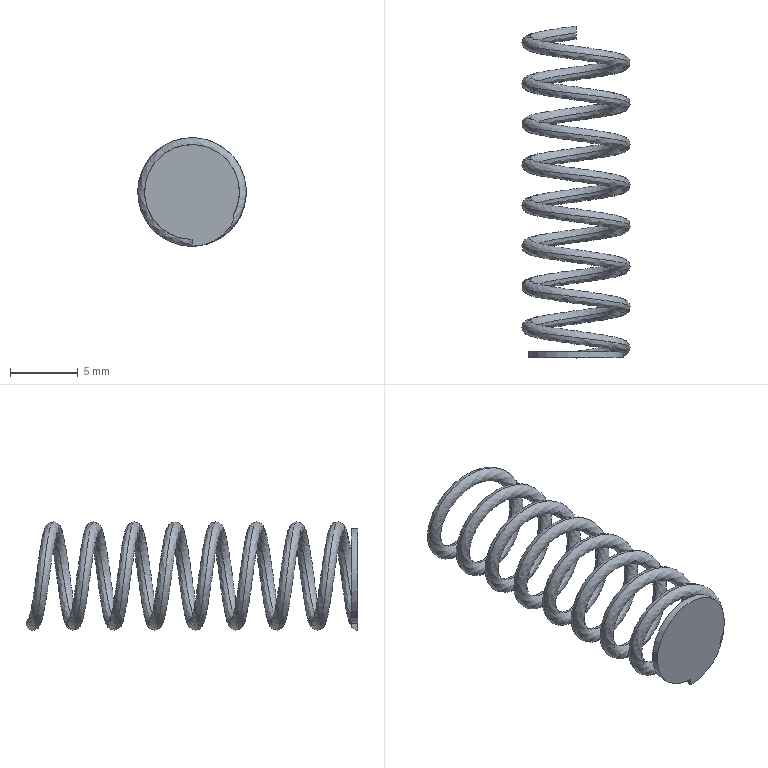Part | STEP file | Round wire coil spring Katalo FUR8-25-B-1 | 1 solid | 7 faces | box 8 x 24.5 x 8 mm | volume 156.394 mm3 | plane 4 | spline 2 | cylinder 1 | commonest cylinder face diameters 7 x1